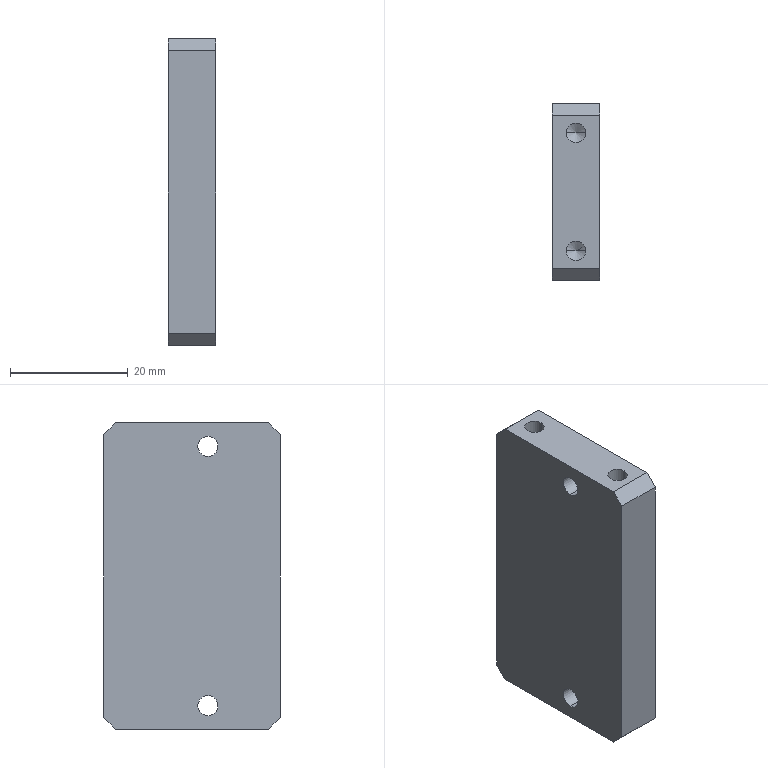Part | STEP file | 11-FG-S02311 | 1 solid | 36 faces | box 8 x 30 x 52 mm | volume 11750 mm3 | cylinder 16 | plane 12 | cone 8 | commonest cylinder face diameters 3.3 x8 3.4 x4 6.5 x4
STEP:
#1=CARTESIAN_POINT('',(-1.65,10.,15.9));
#2=VERTEX_POINT('',#1);
#3=CARTESIAN_POINT('',(1.65,10.,15.9));
#4=VERTEX_POINT('',#3);
#5=CARTESIAN_POINT('',(0.,10.,15.9));
#6=DIRECTION('',(0.,0.,1.));
#7=DIRECTION('',(1.,0.,0.));
#8=AXIS2_PLACEMENT_3D('',#5,#6,#7);
#9=CIRCLE('',#8,1.65);
#10=EDGE_CURVE('',#2,#4,#9,.T.);
#11=ORIENTED_EDGE('',*,*,#10,.F.);
#12=CARTESIAN_POINT('',(-1.65,10.,26.));
#13=VERTEX_POINT('',#12);
#14=CARTESIAN_POINT('',(-1.65,10.,26.));
#15=DIRECTION('',(0.,0.,1.));
#16=VECTOR('',#15,1000.);
#17=LINE('',#14,#16);
#18=EDGE_CURVE('',#2,#13,#17,.T.);
#19=ORIENTED_EDGE('',*,*,#18,.T.);
#20=CARTESIAN_POINT('',(1.65,10.,26.));
#21=VERTEX_POINT('',#20);
#22=CARTESIAN_POINT('',(0.,10.,26.));
#23=DIRECTION('',(0.,0.,1.));
#24=DIRECTION('',(1.,0.,0.));
#25=AXIS2_PLACEMENT_3D('',#22,#23,#24);
#26=CIRCLE('',#25,1.65);
#27=EDGE_CURVE('',#13,#21,#26,.T.);
#28=ORIENTED_EDGE('',*,*,#27,.T.);
#29=CARTESIAN_POINT('',(1.65,10.,26.));
#30=DIRECTION('',(0.,0.,1.));
#31=VECTOR('',#30,1000.);
#32=LINE('',#29,#31);
#33=EDGE_CURVE('',#4,#21,#32,.T.);
#34=ORIENTED_EDGE('',*,*,#33,.F.);
#35=EDGE_LOOP('',(#11,#19,#28,#34));
#36=FACE_OUTER_BOUND('',#35,.T.);
#37=CARTESIAN_POINT('',(0.,10.,26.));
#38=DIRECTION('',(0.,0.,1.));
#39=DIRECTION('',(1.,0.,0.));
#40=AXIS2_PLACEMENT_3D('',#37,#38,#39);
#41=CYLINDRICAL_SURFACE('',#40,1.65);
#42=ADVANCED_FACE('',(#36),#41,.F.);
#43=CARTESIAN_POINT('',(0.,10.,14.909));
#44=VERTEX_POINT('',#43);
#45=CARTESIAN_POINT('',(1.65,10.,15.9));
#46=DIRECTION('',(0.8572,0.,0.515));
#47=VECTOR('',#46,1000.);
#48=LINE('',#45,#47);
#49=EDGE_CURVE('',#44,#4,#48,.T.);
#50=ORIENTED_EDGE('',*,*,#49,.F.);
#51=CARTESIAN_POINT('',(-1.65,10.,15.9));
#52=DIRECTION('',(-0.8572,0.,0.515));
#53=VECTOR('',#52,1000.);
#54=LINE('',#51,#53);
#55=EDGE_CURVE('',#44,#2,#54,.T.);
#56=ORIENTED_EDGE('',*,*,#55,.T.);
#57=ORIENTED_EDGE('',*,*,#10,.T.);
#58=EDGE_LOOP('',(#50,#56,#57));
#59=FACE_OUTER_BOUND('',#58,.T.);
#60=CARTESIAN_POINT('',(0.,10.,15.9));
#61=DIRECTION('',(0.,0.,1.));
#62=DIRECTION('',(1.,0.,0.));
#63=AXIS2_PLACEMENT_3D('',#60,#61,#62);
#64=CONICAL_SURFACE('',#63,1.65,1.03);
#65=ADVANCED_FACE('',(#59),#64,.F.);
#66=CARTESIAN_POINT('',(-1.65,-10.,15.9));
#67=VERTEX_POINT('',#66);
#68=CARTESIAN_POINT('',(1.65,-10.,15.9));
#69=VERTEX_POINT('',#68);
#70=CARTESIAN_POINT('',(0.,-10.,15.9));
#71=DIRECTION('',(0.,0.,1.));
#72=DIRECTION('',(1.,0.,0.));
#73=AXIS2_PLACEMENT_3D('',#70,#71,#72);
#74=CIRCLE('',#73,1.65);
#75=EDGE_CURVE('',#67,#69,#74,.T.);
#76=ORIENTED_EDGE('',*,*,#75,.F.);
#77=CARTESIAN_POINT('',(-1.65,-10.,26.));
#78=VERTEX_POINT('',#77);
#79=CARTESIAN_POINT('',(-1.65,-10.,26.));
#80=DIRECTION('',(0.,0.,1.));
#81=VECTOR('',#80,1000.);
#82=LINE('',#79,#81);
#83=EDGE_CURVE('',#67,#78,#82,.T.);
#84=ORIENTED_EDGE('',*,*,#83,.T.);
#85=CARTESIAN_POINT('',(1.65,-10.,26.));
#86=VERTEX_POINT('',#85);
#87=CARTESIAN_POINT('',(0.,-10.,26.));
#88=DIRECTION('',(0.,0.,1.));
#89=DIRECTION('',(1.,0.,0.));
#90=AXIS2_PLACEMENT_3D('',#87,#88,#89);
#91=CIRCLE('',#90,1.65);
#92=EDGE_CURVE('',#78,#86,#91,.T.);
#93=ORIENTED_EDGE('',*,*,#92,.T.);
#94=CARTESIAN_POINT('',(1.65,-10.,26.));
#95=DIRECTION('',(0.,0.,1.));
#96=VECTOR('',#95,1000.);
#97=LINE('',#94,#96);
#98=EDGE_CURVE('',#69,#86,#97,.T.);
#99=ORIENTED_EDGE('',*,*,#98,.F.);
#100=EDGE_LOOP('',(#76,#84,#93,#99));
#101=FACE_OUTER_BOUND('',#100,.T.);
#102=CARTESIAN_POINT('',(0.,-10.,26.));
#103=DIRECTION('',(0.,0.,1.));
#104=DIRECTION('',(1.,0.,0.));
#105=AXIS2_PLACEMENT_3D('',#102,#103,#104);
#106=CYLINDRICAL_SURFACE('',#105,1.65);
#107=ADVANCED_FACE('',(#101),#106,.F.);
#108=CARTESIAN_POINT('',(0.,-10.,14.909));
#109=VERTEX_POINT('',#108);
#110=CARTESIAN_POINT('',(1.65,-10.,15.9));
#111=DIRECTION('',(0.8572,0.,0.515));
#112=VECTOR('',#111,1000.);
#113=LINE('',#110,#112);
#114=EDGE_CURVE('',#109,#69,#113,.T.);
#115=ORIENTED_EDGE('',*,*,#114,.F.);
#116=CARTESIAN_POINT('',(-1.65,-10.,15.9));
#117=DIRECTION('',(-0.8572,0.,0.515));
#118=VECTOR('',#117,1000.);
#119=LINE('',#116,#118);
#120=EDGE_CURVE('',#109,#67,#119,.T.);
#121=ORIENTED_EDGE('',*,*,#120,.T.);
#122=ORIENTED_EDGE('',*,*,#75,.T.);
#123=EDGE_LOOP('',(#115,#121,#122));
#124=FACE_OUTER_BOUND('',#123,.T.);
#125=CARTESIAN_POINT('',(0.,-10.,15.9));
#126=DIRECTION('',(0.,0.,1.));
#127=DIRECTION('',(1.,0.,0.));
#128=AXIS2_PLACEMENT_3D('',#125,#126,#127);
#129=CONICAL_SURFACE('',#128,1.65,1.03);
#130=ADVANCED_FACE('',(#124),#129,.F.);
#131=CARTESIAN_POINT('',(1.65,10.,-15.9));
#132=VERTEX_POINT('',#131);
#133=CARTESIAN_POINT('',(-1.65,10.,-15.9));
#134=VERTEX_POINT('',#133);
#135=CARTESIAN_POINT('',(0.,10.,-15.9));
#136=DIRECTION('',(0.,0.,-1.));
#137=DIRECTION('',(-1.,0.,0.));
#138=AXIS2_PLACEMENT_3D('',#135,#136,#137);
#139=CIRCLE('',#138,1.65);
#140=EDGE_CURVE('',#132,#134,#139,.T.);
#141=ORIENTED_EDGE('',*,*,#140,.F.);
#142=CARTESIAN_POINT('',(1.65,10.,-26.));
#143=VERTEX_POINT('',#142);
#144=CARTESIAN_POINT('',(1.65,10.,-26.));
#145=DIRECTION('',(0.,0.,-1.));
#146=VECTOR('',#145,1000.);
#147=LINE('',#144,#146);
#148=EDGE_CURVE('',#132,#143,#147,.T.);
#149=ORIENTED_EDGE('',*,*,#148,.T.);
#150=CARTESIAN_POINT('',(-1.65,10.,-26.));
#151=VERTEX_POINT('',#150);
#152=CARTESIAN_POINT('',(0.,10.,-26.));
#153=DIRECTION('',(0.,0.,-1.));
#154=DIRECTION('',(-1.,0.,0.));
#155=AXIS2_PLACEMENT_3D('',#152,#153,#154);
#156=CIRCLE('',#155,1.65);
#157=EDGE_CURVE('',#143,#151,#156,.T.);
#158=ORIENTED_EDGE('',*,*,#157,.T.);
#159=CARTESIAN_POINT('',(-1.65,10.,-26.));
#160=DIRECTION('',(0.,0.,-1.));
#161=VECTOR('',#160,1000.);
#162=LINE('',#159,#161);
#163=EDGE_CURVE('',#134,#151,#162,.T.);
#164=ORIENTED_EDGE('',*,*,#163,.F.);
#165=EDGE_LOOP('',(#141,#149,#158,#164));
#166=FACE_OUTER_BOUND('',#165,.T.);
#167=CARTESIAN_POINT('',(0.,10.,-26.));
#168=DIRECTION('',(0.,0.,-1.));
#169=DIRECTION('',(-1.,0.,0.));
#170=AXIS2_PLACEMENT_3D('',#167,#168,#169);
#171=CYLINDRICAL_SURFACE('',#170,1.65);
#172=ADVANCED_FACE('',(#166),#171,.F.);
#173=CARTESIAN_POINT('',(0.,10.,-14.909));
#174=VERTEX_POINT('',#173);
#175=CARTESIAN_POINT('',(-1.65,10.,-15.9));
#176=DIRECTION('',(-0.8572,0.,-0.515));
#177=VECTOR('',#176,1000.);
#178=LINE('',#175,#177);
#179=EDGE_CURVE('',#174,#134,#178,.T.);
#180=ORIENTED_EDGE('',*,*,#179,.F.);
#181=CARTESIAN_POINT('',(1.65,10.,-15.9));
#182=DIRECTION('',(0.8572,0.,-0.515));
#183=VECTOR('',#182,1000.);
#184=LINE('',#181,#183);
#185=EDGE_CURVE('',#174,#132,#184,.T.);
#186=ORIENTED_EDGE('',*,*,#185,.T.);
#187=ORIENTED_EDGE('',*,*,#140,.T.);
#188=EDGE_LOOP('',(#180,#186,#187));
#189=FACE_OUTER_BOUND('',#188,.T.);
#190=CARTESIAN_POINT('',(0.,10.,-15.9));
#191=DIRECTION('',(0.,0.,-1.));
#192=DIRECTION('',(-1.,0.,0.));
#193=AXIS2_PLACEMENT_3D('',#190,#191,#192);
#194=CONICAL_SURFACE('',#193,1.65,1.03);
#195=ADVANCED_FACE('',(#189),#194,.F.);
#196=CARTESIAN_POINT('',(1.65,-10.,-15.9));
#197=VERTEX_POINT('',#196);
#198=CARTESIAN_POINT('',(-1.65,-10.,-15.9));
#199=VERTEX_POINT('',#198);
#200=CARTESIAN_POINT('',(0.,-10.,-15.9));
#201=DIRECTION('',(0.,0.,-1.));
#202=DIRECTION('',(-1.,0.,0.));
#203=AXIS2_PLACEMENT_3D('',#200,#201,#202);
#204=CIRCLE('',#203,1.65);
#205=EDGE_CURVE('',#197,#199,#204,.T.);
#206=ORIENTED_EDGE('',*,*,#205,.F.);
#207=CARTESIAN_POINT('',(1.65,-10.,-26.));
#208=VERTEX_POINT('',#207);
#209=CARTESIAN_POINT('',(1.65,-10.,-26.));
#210=DIRECTION('',(0.,0.,-1.));
#211=VECTOR('',#210,1000.);
#212=LINE('',#209,#211);
#213=EDGE_CURVE('',#197,#208,#212,.T.);
#214=ORIENTED_EDGE('',*,*,#213,.T.);
#215=CARTESIAN_POINT('',(-1.65,-10.,-26.));
#216=VERTEX_POINT('',#215);
#217=CARTESIAN_POINT('',(0.,-10.,-26.));
#218=DIRECTION('',(0.,0.,-1.));
#219=DIRECTION('',(-1.,0.,0.));
#220=AXIS2_PLACEMENT_3D('',#217,#218,#219);
#221=CIRCLE('',#220,1.65);
#222=EDGE_CURVE('',#208,#216,#221,.T.);
#223=ORIENTED_EDGE('',*,*,#222,.T.);
#224=CARTESIAN_POINT('',(-1.65,-10.,-26.));
#225=DIRECTION('',(0.,0.,-1.));
#226=VECTOR('',#225,1000.);
#227=LINE('',#224,#226);
#228=EDGE_CURVE('',#199,#216,#227,.T.);
#229=ORIENTED_EDGE('',*,*,#228,.F.);
#230=EDGE_LOOP('',(#206,#214,#223,#229));
#231=FACE_OUTER_BOUND('',#230,.T.);
#232=CARTESIAN_POINT('',(0.,-10.,-26.));
#233=DIRECTION('',(0.,0.,-1.));
#234=DIRECTION('',(-1.,0.,0.));
#235=AXIS2_PLACEMENT_3D('',#232,#233,#234);
#236=CYLINDRICAL_SURFACE('',#235,1.65);
#237=ADVANCED_FACE('',(#231),#236,.F.);
#238=CARTESIAN_POINT('',(0.,-10.,-14.909));
#239=VERTEX_POINT('',#238);
#240=CARTESIAN_POINT('',(-1.65,-10.,-15.9));
#241=DIRECTION('',(-0.8572,0.,-0.515));
#242=VECTOR('',#241,1000.);
#243=LINE('',#240,#242);
#244=EDGE_CURVE('',#239,#199,#243,.T.);
#245=ORIENTED_EDGE('',*,*,#244,.F.);
#246=CARTESIAN_POINT('',(1.65,-10.,-15.9));
#247=DIRECTION('',(0.8572,0.,-0.515));
#248=VECTOR('',#247,1000.);
#249=LINE('',#246,#248);
#250=EDGE_CURVE('',#239,#197,#249,.T.);
#251=ORIENTED_EDGE('',*,*,#250,.T.);
#252=ORIENTED_EDGE('',*,*,#205,.T.);
#253=EDGE_LOOP('',(#245,#251,#252));
#254=FACE_OUTER_BOUND('',#253,.T.);
#255=CARTESIAN_POINT('',(0.,-10.,-15.9));
#256=DIRECTION('',(0.,0.,-1.));
#257=DIRECTION('',(-1.,0.,0.));
#258=AXIS2_PLACEMENT_3D('',#255,#256,#257);
#259=CONICAL_SURFACE('',#258,1.65,1.03);
#260=ADVANCED_FACE('',(#254),#259,.F.);
#261=CARTESIAN_POINT('',(0.6,-2.7,-18.75));
#262=VERTEX_POINT('',#261);
#263=CARTESIAN_POINT('',(0.6,-2.7,-25.25));
#264=VERTEX_POINT('',#263);
#265=CARTESIAN_POINT('',(0.6,-2.7,-22.));
#266=DIRECTION('',(1.,0.,0.));
#267=DIRECTION('',(0.,0.,-1.));
#268=AXIS2_PLACEMENT_3D('',#265,#266,#267);
#269=CIRCLE('',#268,3.25);
#270=EDGE_CURVE('',#262,#264,#269,.T.);
#271=ORIENTED_EDGE('',*,*,#270,.F.);
#272=CARTESIAN_POINT('',(4.,-2.7,-18.75));
#273=VERTEX_POINT('',#272);
#274=CARTESIAN_POINT('',(4.,-2.7,-18.75));
#275=DIRECTION('',(1.,0.,0.));
#276=VECTOR('',#275,1000.);
#277=LINE('',#274,#276);
#278=EDGE_CURVE('',#262,#273,#277,.T.);
#279=ORIENTED_EDGE('',*,*,#278,.T.);
#280=CARTESIAN_POINT('',(4.,-2.7,-25.25));
#281=VERTEX_POINT('',#280);
#282=CARTESIAN_POINT('',(4.,-2.7,-22.));
#283=DIRECTION('',(1.,0.,0.));
#284=DIRECTION('',(0.,0.,-1.));
#285=AXIS2_PLACEMENT_3D('',#282,#283,#284);
#286=CIRCLE('',#285,3.25);
#287=EDGE_CURVE('',#273,#281,#286,.T.);
#288=ORIENTED_EDGE('',*,*,#287,.T.);
#289=CARTESIAN_POINT('',(4.,-2.7,-25.25));
#290=DIRECTION('',(1.,0.,0.));
#291=VECTOR('',#290,1000.);
#292=LINE('',#289,#291);
#293=EDGE_CURVE('',#264,#281,#292,.T.);
#294=ORIENTED_EDGE('',*,*,#293,.F.);
#295=EDGE_LOOP('',(#271,#279,#288,#294));
#296=FACE_OUTER_BOUND('',#295,.T.);
#297=CARTESIAN_POINT('',(4.,-2.7,-22.));
#298=DIRECTION('',(1.,0.,0.));
#299=DIRECTION('',(0.,0.,-1.));
#300=AXIS2_PLACEMENT_3D('',#297,#298,#299);
#301=CYLINDRICAL_SURFACE('',#300,3.25);
#302=ADVANCED_FACE('',(#296),#301,.F.);
#303=CARTESIAN_POINT('',(-4.,-2.7,-20.3));
#304=VERTEX_POINT('',#303);
#305=CARTESIAN_POINT('',(-4.,-2.7,-23.7));
#306=VERTEX_POINT('',#305);
#307=CARTESIAN_POINT('',(-4.,-2.7,-22.));
#308=DIRECTION('',(1.,0.,0.));
#309=DIRECTION('',(0.,0.,-1.));
#310=AXIS2_PLACEMENT_3D('',#307,#308,#309);
#311=CIRCLE('',#310,1.7);
#312=EDGE_CURVE('',#304,#306,#311,.T.);
#313=ORIENTED_EDGE('',*,*,#312,.F.);
#314=CARTESIAN_POINT('',(0.6,-2.7,-20.3));
#315=VERTEX_POINT('',#314);
#316=CARTESIAN_POINT('',(4.,-2.7,-20.3));
#317=DIRECTION('',(1.,0.,0.));
#318=VECTOR('',#317,1000.);
#319=LINE('',#316,#318);
#320=EDGE_CURVE('',#304,#315,#319,.T.);
#321=ORIENTED_EDGE('',*,*,#320,.T.);
#322=CARTESIAN_POINT('',(0.6,-2.7,-23.7));
#323=VERTEX_POINT('',#322);
#324=CARTESIAN_POINT('',(0.6,-2.7,-22.));
#325=DIRECTION('',(1.,0.,0.));
#326=DIRECTION('',(0.,0.,-1.));
#327=AXIS2_PLACEMENT_3D('',#324,#325,#326);
#328=CIRCLE('',#327,1.7);
#329=EDGE_CURVE('',#315,#323,#328,.T.);
#330=ORIENTED_EDGE('',*,*,#329,.T.);
#331=CARTESIAN_POINT('',(4.,-2.7,-23.7));
#332=DIRECTION('',(1.,0.,0.));
#333=VECTOR('',#332,1000.);
#334=LINE('',#331,#333);
#335=EDGE_CURVE('',#306,#323,#334,.T.);
#336=ORIENTED_EDGE('',*,*,#335,.F.);
#337=EDGE_LOOP('',(#313,#321,#330,#336));
#338=FACE_OUTER_BOUND('',#337,.T.);
#339=CARTESIAN_POINT('',(4.,-2.7,-22.));
#340=DIRECTION('',(1.,0.,0.));
#341=DIRECTION('',(0.,0.,-1.));
#342=AXIS2_PLACEMENT_3D('',#339,#340,#341);
#343=CYLINDRICAL_SURFACE('',#342,1.7);
#344=ADVANCED_FACE('',(#338),#343,.F.);
#345=CARTESIAN_POINT('',(0.6,-2.7,25.25));
#346=VERTEX_POINT('',#345);
#347=CARTESIAN_POINT('',(0.6,-2.7,18.75));
#348=VERTEX_POINT('',#347);
#349=CARTESIAN_POINT('',(0.6,-2.7,22.));
#350=DIRECTION('',(1.,0.,0.));
#351=DIRECTION('',(0.,0.,-1.));
#352=AXIS2_PLACEMENT_3D('',#349,#350,#351);
#353=CIRCLE('',#352,3.25);
#354=EDGE_CURVE('',#346,#348,#353,.T.);
#355=ORIENTED_EDGE('',*,*,#354,.F.);
#356=CARTESIAN_POINT('',(4.,-2.7,25.25));
#357=VERTEX_POINT('',#356);
#358=CARTESIAN_POINT('',(4.,-2.7,25.25));
#359=DIRECTION('',(1.,0.,0.));
#360=VECTOR('',#359,1000.);
#361=LINE('',#358,#360);
#362=EDGE_CURVE('',#346,#357,#361,.T.);
#363=ORIENTED_EDGE('',*,*,#362,.T.);
#364=CARTESIAN_POINT('',(4.,-2.7,18.75));
#365=VERTEX_POINT('',#364);
#366=CARTESIAN_POINT('',(4.,-2.7,22.));
#367=DIRECTION('',(1.,0.,0.));
#368=DIRECTION('',(0.,0.,-1.));
#369=AXIS2_PLACEMENT_3D('',#366,#367,#368);
#370=CIRCLE('',#369,3.25);
#371=EDGE_CURVE('',#357,#365,#370,.T.);
#372=ORIENTED_EDGE('',*,*,#371,.T.);
#373=CARTESIAN_POINT('',(4.,-2.7,18.75));
#374=DIRECTION('',(1.,0.,0.));
#375=VECTOR('',#374,1000.);
#376=LINE('',#373,#375);
#377=EDGE_CURVE('',#348,#365,#376,.T.);
#378=ORIENTED_EDGE('',*,*,#377,.F.);
#379=EDGE_LOOP('',(#355,#363,#372,#378));
#380=FACE_OUTER_BOUND('',#379,.T.);
#381=CARTESIAN_POINT('',(4.,-2.7,22.));
#382=DIRECTION('',(1.,0.,0.));
#383=DIRECTION('',(0.,0.,-1.));
#384=AXIS2_PLACEMENT_3D('',#381,#382,#383);
#385=CYLINDRICAL_SURFACE('',#384,3.25);
#386=ADVANCED_FACE('',(#380),#385,.F.);
#387=CARTESIAN_POINT('',(-4.,-2.7,23.7));
#388=VERTEX_POINT('',#387);
#389=CARTESIAN_POINT('',(-4.,-2.7,20.3));
#390=VERTEX_POINT('',#389);
#391=CARTESIAN_POINT('',(-4.,-2.7,22.));
#392=DIRECTION('',(1.,0.,0.));
#393=DIRECTION('',(0.,0.,-1.));
#394=AXIS2_PLACEMENT_3D('',#391,#392,#393);
#395=CIRCLE('',#394,1.7);
#396=EDGE_CURVE('',#388,#390,#395,.T.);
#397=ORIENTED_EDGE('',*,*,#396,.F.);
#398=CARTESIAN_POINT('',(0.6,-2.7,23.7));
#399=VERTEX_POINT('',#398);
#400=CARTESIAN_POINT('',(4.,-2.7,23.7));
#401=DIRECTION('',(1.,0.,0.));
#402=VECTOR('',#401,1000.);
#403=LINE('',#400,#402);
#404=EDGE_CURVE('',#388,#399,#403,.T.);
#405=ORIENTED_EDGE('',*,*,#404,.T.);
#406=CARTESIAN_POINT('',(0.6,-2.7,20.3));
#407=VERTEX_POINT('',#406);
#408=CARTESIAN_POINT('',(0.6,-2.7,22.));
#409=DIRECTION('',(1.,0.,0.));
#410=DIRECTION('',(0.,0.,-1.));
#411=AXIS2_PLACEMENT_3D('',#408,#409,#410);
#412=CIRCLE('',#411,1.7);
#413=EDGE_CURVE('',#399,#407,#412,.T.);
#414=ORIENTED_EDGE('',*,*,#413,.T.);
#415=CARTESIAN_POINT('',(4.,-2.7,20.3));
#416=DIRECTION('',(1.,0.,0.));
#417=VECTOR('',#416,1000.);
#418=LINE('',#415,#417);
#419=EDGE_CURVE('',#390,#407,#418,.T.);
#420=ORIENTED_EDGE('',*,*,#419,.F.);
#421=EDGE_LOOP('',(#397,#405,#414,#420));
#422=FACE_OUTER_BOUND('',#421,.T.);
#423=CARTESIAN_POINT('',(4.,-2.7,22.));
#424=DIRECTION('',(1.,0.,0.));
#425=DIRECTION('',(0.,0.,-1.));
#426=AXIS2_PLACEMENT_3D('',#423,#424,#425);
#427=CYLINDRICAL_SURFACE('',#426,1.7);
#428=ADVANCED_FACE('',(#422),#427,.F.);
#429=CARTESIAN_POINT('',(4.,-2.7,-22.));
#430=DIRECTION('',(1.,0.,0.));
#431=DIRECTION('',(0.,0.,-1.));
#432=AXIS2_PLACEMENT_3D('',#429,#430,#431);
#433=CIRCLE('',#432,3.25);
#434=EDGE_CURVE('',#281,#273,#433,.T.);
#435=ORIENTED_EDGE('',*,*,#434,.F.);
#436=ORIENTED_EDGE('',*,*,#287,.F.);
#437=EDGE_LOOP('',(#435,#436));
#438=FACE_BOUND('',#437,.T.);
#439=CARTESIAN_POINT('',(4.,-2.7,22.));
#440=DIRECTION('',(1.,0.,0.));
#441=DIRECTION('',(0.,0.,-1.));
#442=AXIS2_PLACEMENT_3D('',#439,#440,#441);
#443=CIRCLE('',#442,3.25);
#444=EDGE_CURVE('',#365,#357,#443,.T.);
#445=ORIENTED_EDGE('',*,*,#444,.F.);
#446=ORIENTED_EDGE('',*,*,#371,.F.);
#447=EDGE_LOOP('',(#445,#446));
#448=FACE_BOUND('',#447,.T.);
#449=CARTESIAN_POINT('',(4.,15.,24.));
#450=VERTEX_POINT('',#449);
#451=CARTESIAN_POINT('',(4.,15.,-24.));
#452=VERTEX_POINT('',#451);
#453=CARTESIAN_POINT('',(4.,15.,26.));
#454=DIRECTION('',(0.,0.,-1.));
#455=VECTOR('',#454,1000.);
#456=LINE('',#453,#455);
#457=EDGE_CURVE('',#450,#452,#456,.T.);
#458=ORIENTED_EDGE('',*,*,#457,.F.);
#459=CARTESIAN_POINT('',(4.,13.,26.));
#460=VERTEX_POINT('',#459);
#461=CARTESIAN_POINT('',(4.,13.,26.));
#462=DIRECTION('',(0.,-0.7071,0.7071));
#463=VECTOR('',#462,1000.);
#464=LINE('',#461,#463);
#465=EDGE_CURVE('',#450,#460,#464,.T.);
#466=ORIENTED_EDGE('',*,*,#465,.T.);
#467=CARTESIAN_POINT('',(4.,-13.,26.));
#468=VERTEX_POINT('',#467);
#469=CARTESIAN_POINT('',(4.,-15.,26.));
#470=DIRECTION('',(0.,1.,0.));
#471=VECTOR('',#470,1000.);
#472=LINE('',#469,#471);
#473=EDGE_CURVE('',#468,#460,#472,.T.);
#474=ORIENTED_EDGE('',*,*,#473,.F.);
#475=CARTESIAN_POINT('',(4.,-15.,24.));
#476=VERTEX_POINT('',#475);
#477=CARTESIAN_POINT('',(4.,-13.,26.));
#478=DIRECTION('',(0.,-0.7071,-0.7071));
#479=VECTOR('',#478,1000.);
#480=LINE('',#477,#479);
#481=EDGE_CURVE('',#468,#476,#480,.T.);
#482=ORIENTED_EDGE('',*,*,#481,.T.);
#483=CARTESIAN_POINT('',(4.,-15.,-24.));
#484=VERTEX_POINT('',#483);
#485=CARTESIAN_POINT('',(4.,-15.,26.));
#486=DIRECTION('',(0.,0.,-1.));
#487=VECTOR('',#486,1000.);
#488=LINE('',#485,#487);
#489=EDGE_CURVE('',#476,#484,#488,.T.);
#490=ORIENTED_EDGE('',*,*,#489,.T.);
#491=CARTESIAN_POINT('',(4.,-13.,-26.));
#492=VERTEX_POINT('',#491);
#493=CARTESIAN_POINT('',(4.,-15.,-24.));
#494=DIRECTION('',(0.,0.7071,-0.7071));
#495=VECTOR('',#494,1000.);
#496=LINE('',#493,#495);
#497=EDGE_CURVE('',#484,#492,#496,.T.);
#498=ORIENTED_EDGE('',*,*,#497,.T.);
#499=CARTESIAN_POINT('',(4.,13.,-26.));
#500=VERTEX_POINT('',#499);
#501=CARTESIAN_POINT('',(4.,-15.,-26.));
#502=DIRECTION('',(0.,1.,0.));
#503=VECTOR('',#502,1000.);
#504=LINE('',#501,#503);
#505=EDGE_CURVE('',#492,#500,#504,.T.);
#506=ORIENTED_EDGE('',*,*,#505,.T.);
#507=CARTESIAN_POINT('',(4.,15.,-24.));
#508=DIRECTION('',(0.,0.7071,0.7071));
#509=VECTOR('',#508,1000.);
#510=LINE('',#507,#509);
#511=EDGE_CURVE('',#500,#452,#510,.T.);
#512=ORIENTED_EDGE('',*,*,#511,.T.);
#513=EDGE_LOOP('',(#458,#466,#474,#482,#490,#498,#506,#512));
#514=FACE_OUTER_BOUND('',#513,.T.);
#515=CARTESIAN_POINT('',(4.,-15.,26.));
#516=DIRECTION('',(-1.,0.,0.));
#517=DIRECTION('',(0.,0.,1.));
#518=AXIS2_PLACEMENT_3D('',#515,#516,#517);
#519=PLANE('',#518);
#520=ADVANCED_FACE('',(#438,#448,#514),#519,.F.);
#521=CARTESIAN_POINT('',(-4.,15.,24.));
#522=VERTEX_POINT('',#521);
#523=CARTESIAN_POINT('',(-4.,15.,-24.));
#524=VERTEX_POINT('',#523);
#525=CARTESIAN_POINT('',(-4.,15.,26.));
#526=DIRECTION('',(0.,0.,-1.));
#527=VECTOR('',#526,1000.);
#528=LINE('',#525,#527);
#529=EDGE_CURVE('',#522,#524,#528,.T.);
#530=ORIENTED_EDGE('',*,*,#529,.F.);
#531=CARTESIAN_POINT('',(-4.,15.,24.));
#532=DIRECTION('',(1.,0.,0.));
#533=VECTOR('',#532,1000.);
#534=LINE('',#531,#533);
#535=EDGE_CURVE('',#522,#450,#534,.T.);
#536=ORIENTED_EDGE('',*,*,#535,.T.);
#537=ORIENTED_EDGE('',*,*,#457,.T.);
#538=CARTESIAN_POINT('',(-4.,15.,-24.));
#539=DIRECTION('',(-1.,0.,0.));
#540=VECTOR('',#539,1000.);
#541=LINE('',#538,#540);
#542=EDGE_CURVE('',#452,#524,#541,.T.);
#543=ORIENTED_EDGE('',*,*,#542,.T.);
#544=EDGE_LOOP('',(#530,#536,#537,#543));
#545=FACE_OUTER_BOUND('',#544,.T.);
#546=CARTESIAN_POINT('',(-4.,15.,26.));
#547=DIRECTION('',(0.,-1.,0.));
#548=DIRECTION('',(0.,0.,-1.));
#549=AXIS2_PLACEMENT_3D('',#546,#547,#548);
#550=PLANE('',#549);
#551=ADVANCED_FACE('',(#545),#550,.F.);
#552=CARTESIAN_POINT('',(-4.,-2.7,-22.));
#553=DIRECTION('',(1.,0.,0.));
#554=DIRECTION('',(0.,0.,-1.));
#555=AXIS2_PLACEMENT_3D('',#552,#553,#554);
#556=CIRCLE('',#555,1.7);
#557=EDGE_CURVE('',#306,#304,#556,.T.);
#558=ORIENTED_EDGE('',*,*,#557,.T.);
#559=ORIENTED_EDGE('',*,*,#312,.T.);
#560=EDGE_LOOP('',(#558,#559));
#561=FACE_BOUND('',#560,.T.);
#562=CARTESIAN_POINT('',(-4.,-2.7,22.));
#563=DIRECTION('',(1.,0.,0.));
#564=DIRECTION('',(0.,0.,-1.));
#565=AXIS2_PLACEMENT_3D('',#562,#563,#564);
#566=CIRCLE('',#565,1.7);
#567=EDGE_CURVE('',#390,#388,#566,.T.);
#568=ORIENTED_EDGE('',*,*,#567,.T.);
#569=ORIENTED_EDGE('',*,*,#396,.T.);
#570=EDGE_LOOP('',(#568,#569));
#571=FACE_BOUND('',#570,.T.);
#572=CARTESIAN_POINT('',(-4.,13.,26.));
#573=VERTEX_POINT('',#572);
#574=CARTESIAN_POINT('',(-4.,-13.,26.));
#575=VERTEX_POINT('',#574);
#576=CARTESIAN_POINT('',(-4.,-15.,26.));
#577=DIRECTION('',(0.,-1.,0.));
#578=VECTOR('',#577,1000.);
#579=LINE('',#576,#578);
#580=EDGE_CURVE('',#573,#575,#579,.T.);
#581=ORIENTED_EDGE('',*,*,#580,.F.);
#582=CARTESIAN_POINT('',(-4.,13.,26.));
#583=DIRECTION('',(0.,0.7071,-0.7071));
#584=VECTOR('',#583,1000.);
#585=LINE('',#582,#584);
#586=EDGE_CURVE('',#573,#522,#585,.T.);
#587=ORIENTED_EDGE('',*,*,#586,.T.);
#588=ORIENTED_EDGE('',*,*,#529,.T.);
#589=CARTESIAN_POINT('',(-4.,13.,-26.));
#590=VERTEX_POINT('',#589);
#591=CARTESIAN_POINT('',(-4.,15.,-24.));
#592=DIRECTION('',(0.,-0.7071,-0.7071));
#593=VECTOR('',#592,1000.);
#594=LINE('',#591,#593);
#595=EDGE_CURVE('',#524,#590,#594,.T.);
#596=ORIENTED_EDGE('',*,*,#595,.T.);
#597=CARTESIAN_POINT('',(-4.,-13.,-26.));
#598=VERTEX_POINT('',#597);
#599=CARTESIAN_POINT('',(-4.,-15.,-26.));
#600=DIRECTION('',(0.,-1.,0.));
#601=VECTOR('',#600,1000.);
#602=LINE('',#599,#601);
#603=EDGE_CURVE('',#590,#598,#602,.T.);
#604=ORIENTED_EDGE('',*,*,#603,.T.);
#605=CARTESIAN_POINT('',(-4.,-15.,-24.));
#606=VERTEX_POINT('',#605);
#607=CARTESIAN_POINT('',(-4.,-15.,-24.));
#608=DIRECTION('',(0.,-0.7071,0.7071));
#609=VECTOR('',#608,1000.);
#610=LINE('',#607,#609);
#611=EDGE_CURVE('',#598,#606,#610,.T.);
#612=ORIENTED_EDGE('',*,*,#611,.T.);
#613=CARTESIAN_POINT('',(-4.,-15.,24.));
#614=VERTEX_POINT('',#613);
#615=CARTESIAN_POINT('',(-4.,-15.,26.));
#616=DIRECTION('',(0.,0.,-1.));
#617=VECTOR('',#616,1000.);
#618=LINE('',#615,#617);
#619=EDGE_CURVE('',#614,#606,#618,.T.);
#620=ORIENTED_EDGE('',*,*,#619,.F.);
#621=CARTESIAN_POINT('',(-4.,-13.,26.));
#622=DIRECTION('',(0.,0.7071,0.7071));
#623=VECTOR('',#622,1000.);
#624=LINE('',#621,#623);
#625=EDGE_CURVE('',#614,#575,#624,.T.);
#626=ORIENTED_EDGE('',*,*,#625,.T.);
#627=EDGE_LOOP('',(#581,#587,#588,#596,#604,#612,#620,#626));
#628=FACE_OUTER_BOUND('',#627,.T.);
#629=CARTESIAN_POINT('',(-4.,-15.,26.));
#630=DIRECTION('',(1.,0.,0.));
#631=DIRECTION('',(0.,0.,-1.));
#632=AXIS2_PLACEMENT_3D('',#629,#630,#631);
#633=PLANE('',#632);
#634=ADVANCED_FACE('',(#561,#571,#628),#633,.F.);
#635=ORIENTED_EDGE('',*,*,#489,.F.);
#636=CARTESIAN_POINT('',(-4.,-15.,24.));
#637=DIRECTION('',(-1.,0.,0.));
#638=VECTOR('',#637,1000.);
#639=LINE('',#636,#638);
#640=EDGE_CURVE('',#476,#614,#639,.T.);
#641=ORIENTED_EDGE('',*,*,#640,.T.);
#642=ORIENTED_EDGE('',*,*,#619,.T.);
#643=CARTESIAN_POINT('',(4.,-15.,-24.));
#644=DIRECTION('',(1.,0.,0.));
#645=VECTOR('',#644,1000.);
#646=LINE('',#643,#645);
#647=EDGE_CURVE('',#606,#484,#646,.T.);
#648=ORIENTED_EDGE('',*,*,#647,.T.);
#649=EDGE_LOOP('',(#635,#641,#642,#648));
#650=FACE_OUTER_BOUND('',#649,.T.);
#651=CARTESIAN_POINT('',(-4.,-15.,26.));
#652=DIRECTION('',(0.,1.,0.));
#653=DIRECTION('',(0.,0.,1.));
#654=AXIS2_PLACEMENT_3D('',#651,#652,#653);
#655=PLANE('',#654);
#656=ADVANCED_FACE('',(#650),#655,.F.);
#657=CARTESIAN_POINT('',(0.,10.,26.));
#658=DIRECTION('',(0.,0.,1.));
#659=DIRECTION('',(1.,0.,0.));
#660=AXIS2_PLACEMENT_3D('',#657,#658,#659);
#661=CIRCLE('',#660,1.65);
#662=EDGE_CURVE('',#21,#13,#661,.T.);
#663=ORIENTED_EDGE('',*,*,#662,.F.);
#664=ORIENTED_EDGE('',*,*,#27,.F.);
#665=EDGE_LOOP('',(#663,#664));
#666=FACE_BOUND('',#665,.T.);
#667=CARTESIAN_POINT('',(0.,-10.,26.));
#668=DIRECTION('',(0.,0.,1.));
#669=DIRECTION('',(1.,0.,0.));
#670=AXIS2_PLACEMENT_3D('',#667,#668,#669);
#671=CIRCLE('',#670,1.65);
#672=EDGE_CURVE('',#86,#78,#671,.T.);
#673=ORIENTED_EDGE('',*,*,#672,.F.);
#674=ORIENTED_EDGE('',*,*,#92,.F.);
#675=EDGE_LOOP('',(#673,#674));
#676=FACE_BOUND('',#675,.T.);
#677=ORIENTED_EDGE('',*,*,#473,.T.);
#678=CARTESIAN_POINT('',(0.,13.,26.));
#679=DIRECTION('',(-1.,0.,0.));
#680=VECTOR('',#679,1000.);
#681=LINE('',#678,#680);
#682=EDGE_CURVE('',#460,#573,#681,.T.);
#683=ORIENTED_EDGE('',*,*,#682,.T.);
#684=ORIENTED_EDGE('',*,*,#580,.T.);
#685=CARTESIAN_POINT('',(0.,-13.,26.));
#686=DIRECTION('',(1.,0.,0.));
#687=VECTOR('',#686,1000.);
#688=LINE('',#685,#687);
#689=EDGE_CURVE('',#575,#468,#688,.T.);
#690=ORIENTED_EDGE('',*,*,#689,.T.);
#691=EDGE_LOOP('',(#677,#683,#684,#690));
#692=FACE_OUTER_BOUND('',#691,.T.);
#693=CARTESIAN_POINT('',(0.,0.,26.));
#694=DIRECTION('',(0.,0.,-1.));
#695=DIRECTION('',(-1.,0.,0.));
#696=AXIS2_PLACEMENT_3D('',#693,#694,#695);
#697=PLANE('',#696);
#698=ADVANCED_FACE('',(#666,#676,#692),#697,.F.);
#699=CARTESIAN_POINT('',(0.,10.,-26.));
#700=DIRECTION('',(0.,0.,-1.));
#701=DIRECTION('',(-1.,0.,0.));
#702=AXIS2_PLACEMENT_3D('',#699,#700,#701);
#703=CIRCLE('',#702,1.65);
#704=EDGE_CURVE('',#151,#143,#703,.T.);
#705=ORIENTED_EDGE('',*,*,#704,.F.);
#706=ORIENTED_EDGE('',*,*,#157,.F.);
#707=EDGE_LOOP('',(#705,#706));
#708=FACE_BOUND('',#707,.T.);
#709=CARTESIAN_POINT('',(0.,-10.,-26.));
#710=DIRECTION('',(0.,0.,-1.));
#711=DIRECTION('',(-1.,0.,0.));
#712=AXIS2_PLACEMENT_3D('',#709,#710,#711);
#713=CIRCLE('',#712,1.65);
#714=EDGE_CURVE('',#216,#208,#713,.T.);
#715=ORIENTED_EDGE('',*,*,#714,.F.);
#716=ORIENTED_EDGE('',*,*,#222,.F.);
#717=EDGE_LOOP('',(#715,#716));
#718=FACE_BOUND('',#717,.T.);
#719=ORIENTED_EDGE('',*,*,#603,.F.);
#720=CARTESIAN_POINT('',(4.,13.,-26.));
#721=DIRECTION('',(1.,0.,0.));
#722=VECTOR('',#721,1000.);
#723=LINE('',#720,#722);
#724=EDGE_CURVE('',#590,#500,#723,.T.);
#725=ORIENTED_EDGE('',*,*,#724,.T.);
#726=ORIENTED_EDGE('',*,*,#505,.F.);
#727=CARTESIAN_POINT('',(-4.,-13.,-26.));
#728=DIRECTION('',(-1.,0.,0.));
#729=VECTOR('',#728,1000.);
#730=LINE('',#727,#729);
#731=EDGE_CURVE('',#492,#598,#730,.T.);
#732=ORIENTED_EDGE('',*,*,#731,.T.);
#733=EDGE_LOOP('',(#719,#725,#726,#732));
#734=FACE_OUTER_BOUND('',#733,.T.);
#735=CARTESIAN_POINT('',(0.,0.,-26.));
#736=DIRECTION('',(0.,0.,-1.));
#737=DIRECTION('',(-1.,0.,0.));
#738=AXIS2_PLACEMENT_3D('',#735,#736,#737);
#739=PLANE('',#738);
#740=ADVANCED_FACE('',(#708,#718,#734),#739,.T.);
#741=ORIENTED_EDGE('',*,*,#404,.F.);
#742=ORIENTED_EDGE('',*,*,#567,.F.);
#743=ORIENTED_EDGE('',*,*,#419,.T.);
#744=CARTESIAN_POINT('',(0.6,-2.7,22.));
#745=DIRECTION('',(1.,0.,0.));
#746=DIRECTION('',(0.,0.,-1.));
#747=AXIS2_PLACEMENT_3D('',#744,#745,#746);
#748=CIRCLE('',#747,1.7);
#749=EDGE_CURVE('',#407,#399,#748,.T.);
#750=ORIENTED_EDGE('',*,*,#749,.T.);
#751=EDGE_LOOP('',(#741,#742,#743,#750));
#752=FACE_OUTER_BOUND('',#751,.T.);
#753=CARTESIAN_POINT('',(4.,-2.7,22.));
#754=DIRECTION('',(1.,0.,0.));
#755=DIRECTION('',(0.,0.,-1.));
#756=AXIS2_PLACEMENT_3D('',#753,#754,#755);
#757=CYLINDRICAL_SURFACE('',#756,1.7);
#758=ADVANCED_FACE('',(#752),#757,.F.);
#759=ORIENTED_EDGE('',*,*,#749,.F.);
#760=ORIENTED_EDGE('',*,*,#413,.F.);
#761=EDGE_LOOP('',(#759,#760));
#762=FACE_BOUND('',#761,.T.);
#763=CARTESIAN_POINT('',(0.6,-2.7,22.));
#764=DIRECTION('',(1.,0.,0.));
#765=DIRECTION('',(0.,0.,-1.));
#766=AXIS2_PLACEMENT_3D('',#763,#764,#765);
#767=CIRCLE('',#766,3.25);
#768=EDGE_CURVE('',#348,#346,#767,.T.);
#769=ORIENTED_EDGE('',*,*,#768,.T.);
#770=ORIENTED_EDGE('',*,*,#354,.T.);
#771=EDGE_LOOP('',(#769,#770));
#772=FACE_OUTER_BOUND('',#771,.T.);
#773=CARTESIAN_POINT('',(0.6,-1.,22.));
#774=DIRECTION('',(-1.,0.,0.));
#775=DIRECTION('',(0.,0.,1.));
#776=AXIS2_PLACEMENT_3D('',#773,#774,#775);
#777=PLANE('',#776);
#778=ADVANCED_FACE('',(#762,#772),#777,.F.);
#779=ORIENTED_EDGE('',*,*,#362,.F.);
#780=ORIENTED_EDGE('',*,*,#768,.F.);
#781=ORIENTED_EDGE('',*,*,#377,.T.);
#782=ORIENTED_EDGE('',*,*,#444,.T.);
#783=EDGE_LOOP('',(#779,#780,#781,#782));
#784=FACE_OUTER_BOUND('',#783,.T.);
#785=CARTESIAN_POINT('',(4.,-2.7,22.));
#786=DIRECTION('',(1.,0.,0.));
#787=DIRECTION('',(0.,0.,-1.));
#788=AXIS2_PLACEMENT_3D('',#785,#786,#787);
#789=CYLINDRICAL_SURFACE('',#788,3.25);
#790=ADVANCED_FACE('',(#784),#789,.F.);
#791=ORIENTED_EDGE('',*,*,#320,.F.);
#792=ORIENTED_EDGE('',*,*,#557,.F.);
#793=ORIENTED_EDGE('',*,*,#335,.T.);
#794=CARTESIAN_POINT('',(0.6,-2.7,-22.));
#795=DIRECTION('',(1.,0.,0.));
#796=DIRECTION('',(0.,0.,-1.));
#797=AXIS2_PLACEMENT_3D('',#794,#795,#796);
#798=CIRCLE('',#797,1.7);
#799=EDGE_CURVE('',#323,#315,#798,.T.);
#800=ORIENTED_EDGE('',*,*,#799,.T.);
#801=EDGE_LOOP('',(#791,#792,#793,#800));
#802=FACE_OUTER_BOUND('',#801,.T.);
#803=CARTESIAN_POINT('',(4.,-2.7,-22.));
#804=DIRECTION('',(1.,0.,0.));
#805=DIRECTION('',(0.,0.,-1.));
#806=AXIS2_PLACEMENT_3D('',#803,#804,#805);
#807=CYLINDRICAL_SURFACE('',#806,1.7);
#808=ADVANCED_FACE('',(#802),#807,.F.);
#809=ORIENTED_EDGE('',*,*,#799,.F.);
#810=ORIENTED_EDGE('',*,*,#329,.F.);
#811=EDGE_LOOP('',(#809,#810));
#812=FACE_BOUND('',#811,.T.);
#813=CARTESIAN_POINT('',(0.6,-2.7,-22.));
#814=DIRECTION('',(1.,0.,0.));
#815=DIRECTION('',(0.,0.,-1.));
#816=AXIS2_PLACEMENT_3D('',#813,#814,#815);
#817=CIRCLE('',#816,3.25);
#818=EDGE_CURVE('',#264,#262,#817,.T.);
#819=ORIENTED_EDGE('',*,*,#818,.T.);
#820=ORIENTED_EDGE('',*,*,#270,.T.);
#821=EDGE_LOOP('',(#819,#820));
#822=FACE_OUTER_BOUND('',#821,.T.);
#823=CARTESIAN_POINT('',(0.6,-1.,-22.));
#824=DIRECTION('',(-1.,0.,0.));
#825=DIRECTION('',(0.,0.,1.));
#826=AXIS2_PLACEMENT_3D('',#823,#824,#825);
#827=PLANE('',#826);
#828=ADVANCED_FACE('',(#812,#822),#827,.F.);
#829=ORIENTED_EDGE('',*,*,#278,.F.);
#830=ORIENTED_EDGE('',*,*,#818,.F.);
#831=ORIENTED_EDGE('',*,*,#293,.T.);
#832=ORIENTED_EDGE('',*,*,#434,.T.);
#833=EDGE_LOOP('',(#829,#830,#831,#832));
#834=FACE_OUTER_BOUND('',#833,.T.);
#835=CARTESIAN_POINT('',(4.,-2.7,-22.));
#836=DIRECTION('',(1.,0.,0.));
#837=DIRECTION('',(0.,0.,-1.));
#838=AXIS2_PLACEMENT_3D('',#835,#836,#837);
#839=CYLINDRICAL_SURFACE('',#838,3.25);
#840=ADVANCED_FACE('',(#834),#839,.F.);
#841=ORIENTED_EDGE('',*,*,#465,.F.);
#842=ORIENTED_EDGE('',*,*,#535,.F.);
#843=ORIENTED_EDGE('',*,*,#586,.F.);
#844=ORIENTED_EDGE('',*,*,#682,.F.);
#845=EDGE_LOOP('',(#841,#842,#843,#844));
#846=FACE_OUTER_BOUND('',#845,.T.);
#847=CARTESIAN_POINT('',(0.,13.,26.));
#848=DIRECTION('',(0.,-0.7071,-0.7071));
#849=DIRECTION('',(-1.,0.,0.));
#850=AXIS2_PLACEMENT_3D('',#847,#848,#849);
#851=PLANE('',#850);
#852=ADVANCED_FACE('',(#846),#851,.F.);
#853=ORIENTED_EDGE('',*,*,#511,.F.);
#854=ORIENTED_EDGE('',*,*,#724,.F.);
#855=ORIENTED_EDGE('',*,*,#595,.F.);
#856=ORIENTED_EDGE('',*,*,#542,.F.);
#857=EDGE_LOOP('',(#853,#854,#855,#856));
#858=FACE_OUTER_BOUND('',#857,.T.);
#859=CARTESIAN_POINT('',(-4.,15.,-24.));
#860=DIRECTION('',(0.,0.7071,-0.7071));
#861=DIRECTION('',(1.,0.,0.));
#862=AXIS2_PLACEMENT_3D('',#859,#860,#861);
#863=PLANE('',#862);
#864=ADVANCED_FACE('',(#858),#863,.T.);
#865=ORIENTED_EDGE('',*,*,#625,.F.);
#866=ORIENTED_EDGE('',*,*,#640,.F.);
#867=ORIENTED_EDGE('',*,*,#481,.F.);
#868=ORIENTED_EDGE('',*,*,#689,.F.);
#869=EDGE_LOOP('',(#865,#866,#867,#868));
#870=FACE_OUTER_BOUND('',#869,.T.);
#871=CARTESIAN_POINT('',(0.,-13.,26.));
#872=DIRECTION('',(0.,0.7071,-0.7071));
#873=DIRECTION('',(1.,0.,0.));
#874=AXIS2_PLACEMENT_3D('',#871,#872,#873);
#875=PLANE('',#874);
#876=ADVANCED_FACE('',(#870),#875,.F.);
#877=ORIENTED_EDGE('',*,*,#611,.F.);
#878=ORIENTED_EDGE('',*,*,#731,.F.);
#879=ORIENTED_EDGE('',*,*,#497,.F.);
#880=ORIENTED_EDGE('',*,*,#647,.F.);
#881=EDGE_LOOP('',(#877,#878,#879,#880));
#882=FACE_OUTER_BOUND('',#881,.T.);
#883=CARTESIAN_POINT('',(-4.,-15.,-24.));
#884=DIRECTION('',(0.,-0.7071,-0.7071));
#885=DIRECTION('',(-1.,0.,0.));
#886=AXIS2_PLACEMENT_3D('',#883,#884,#885);
#887=PLANE('',#886);
#888=ADVANCED_FACE('',(#882),#887,.T.);
#889=ORIENTED_EDGE('',*,*,#250,.F.);
#890=ORIENTED_EDGE('',*,*,#244,.T.);
#891=CARTESIAN_POINT('',(0.,-10.,-15.9));
#892=DIRECTION('',(0.,0.,-1.));
#893=DIRECTION('',(-1.,0.,0.));
#894=AXIS2_PLACEMENT_3D('',#891,#892,#893);
#895=CIRCLE('',#894,1.65);
#896=EDGE_CURVE('',#199,#197,#895,.T.);
#897=ORIENTED_EDGE('',*,*,#896,.T.);
#898=EDGE_LOOP('',(#889,#890,#897));
#899=FACE_OUTER_BOUND('',#898,.T.);
#900=CARTESIAN_POINT('',(0.,-10.,-15.9));
#901=DIRECTION('',(0.,0.,-1.));
#902=DIRECTION('',(-1.,0.,0.));
#903=AXIS2_PLACEMENT_3D('',#900,#901,#902);
#904=CONICAL_SURFACE('',#903,1.65,1.03);
#905=ADVANCED_FACE('',(#899),#904,.F.);
#906=ORIENTED_EDGE('',*,*,#213,.F.);
#907=ORIENTED_EDGE('',*,*,#896,.F.);
#908=ORIENTED_EDGE('',*,*,#228,.T.);
#909=ORIENTED_EDGE('',*,*,#714,.T.);
#910=EDGE_LOOP('',(#906,#907,#908,#909));
#911=FACE_OUTER_BOUND('',#910,.T.);
#912=CARTESIAN_POINT('',(0.,-10.,-26.));
#913=DIRECTION('',(0.,0.,-1.));
#914=DIRECTION('',(-1.,0.,0.));
#915=AXIS2_PLACEMENT_3D('',#912,#913,#914);
#916=CYLINDRICAL_SURFACE('',#915,1.65);
#917=ADVANCED_FACE('',(#911),#916,.F.);
#918=ORIENTED_EDGE('',*,*,#185,.F.);
#919=ORIENTED_EDGE('',*,*,#179,.T.);
#920=CARTESIAN_POINT('',(0.,10.,-15.9));
#921=DIRECTION('',(0.,0.,-1.));
#922=DIRECTION('',(-1.,0.,0.));
#923=AXIS2_PLACEMENT_3D('',#920,#921,#922);
#924=CIRCLE('',#923,1.65);
#925=EDGE_CURVE('',#134,#132,#924,.T.);
#926=ORIENTED_EDGE('',*,*,#925,.T.);
#927=EDGE_LOOP('',(#918,#919,#926));
#928=FACE_OUTER_BOUND('',#927,.T.);
#929=CARTESIAN_POINT('',(0.,10.,-15.9));
#930=DIRECTION('',(0.,0.,-1.));
#931=DIRECTION('',(-1.,0.,0.));
#932=AXIS2_PLACEMENT_3D('',#929,#930,#931);
#933=CONICAL_SURFACE('',#932,1.65,1.03);
#934=ADVANCED_FACE('',(#928),#933,.F.);
#935=ORIENTED_EDGE('',*,*,#148,.F.);
#936=ORIENTED_EDGE('',*,*,#925,.F.);
#937=ORIENTED_EDGE('',*,*,#163,.T.);
#938=ORIENTED_EDGE('',*,*,#704,.T.);
#939=EDGE_LOOP('',(#935,#936,#937,#938));
#940=FACE_OUTER_BOUND('',#939,.T.);
#941=CARTESIAN_POINT('',(0.,10.,-26.));
#942=DIRECTION('',(0.,0.,-1.));
#943=DIRECTION('',(-1.,0.,0.));
#944=AXIS2_PLACEMENT_3D('',#941,#942,#943);
#945=CYLINDRICAL_SURFACE('',#944,1.65);
#946=ADVANCED_FACE('',(#940),#945,.F.);
#947=ORIENTED_EDGE('',*,*,#120,.F.);
#948=ORIENTED_EDGE('',*,*,#114,.T.);
#949=CARTESIAN_POINT('',(0.,-10.,15.9));
#950=DIRECTION('',(0.,0.,1.));
#951=DIRECTION('',(1.,0.,0.));
#952=AXIS2_PLACEMENT_3D('',#949,#950,#951);
#953=CIRCLE('',#952,1.65);
#954=EDGE_CURVE('',#69,#67,#953,.T.);
#955=ORIENTED_EDGE('',*,*,#954,.T.);
#956=EDGE_LOOP('',(#947,#948,#955));
#957=FACE_OUTER_BOUND('',#956,.T.);
#958=CARTESIAN_POINT('',(0.,-10.,15.9));
#959=DIRECTION('',(0.,0.,1.));
#960=DIRECTION('',(1.,0.,0.));
#961=AXIS2_PLACEMENT_3D('',#958,#959,#960);
#962=CONICAL_SURFACE('',#961,1.65,1.03);
#963=ADVANCED_FACE('',(#957),#962,.F.);
#964=ORIENTED_EDGE('',*,*,#83,.F.);
#965=ORIENTED_EDGE('',*,*,#954,.F.);
#966=ORIENTED_EDGE('',*,*,#98,.T.);
#967=ORIENTED_EDGE('',*,*,#672,.T.);
#968=EDGE_LOOP('',(#964,#965,#966,#967));
#969=FACE_OUTER_BOUND('',#968,.T.);
#970=CARTESIAN_POINT('',(0.,-10.,26.));
#971=DIRECTION('',(0.,0.,1.));
#972=DIRECTION('',(1.,0.,0.));
#973=AXIS2_PLACEMENT_3D('',#970,#971,#972);
#974=CYLINDRICAL_SURFACE('',#973,1.65);
#975=ADVANCED_FACE('',(#969),#974,.F.);
#976=ORIENTED_EDGE('',*,*,#55,.F.);
#977=ORIENTED_EDGE('',*,*,#49,.T.);
#978=CARTESIAN_POINT('',(0.,10.,15.9));
#979=DIRECTION('',(0.,0.,1.));
#980=DIRECTION('',(1.,0.,0.));
#981=AXIS2_PLACEMENT_3D('',#978,#979,#980);
#982=CIRCLE('',#981,1.65);
#983=EDGE_CURVE('',#4,#2,#982,.T.);
#984=ORIENTED_EDGE('',*,*,#983,.T.);
#985=EDGE_LOOP('',(#976,#977,#984));
#986=FACE_OUTER_BOUND('',#985,.T.);
#987=CARTESIAN_POINT('',(0.,10.,15.9));
#988=DIRECTION('',(0.,0.,1.));
#989=DIRECTION('',(1.,0.,0.));
#990=AXIS2_PLACEMENT_3D('',#987,#988,#989);
#991=CONICAL_SURFACE('',#990,1.65,1.03);
#992=ADVANCED_FACE('',(#986),#991,.F.);
#993=ORIENTED_EDGE('',*,*,#18,.F.);
#994=ORIENTED_EDGE('',*,*,#983,.F.);
#995=ORIENTED_EDGE('',*,*,#33,.T.);
#996=ORIENTED_EDGE('',*,*,#662,.T.);
#997=EDGE_LOOP('',(#993,#994,#995,#996));
#998=FACE_OUTER_BOUND('',#997,.T.);
#999=CARTESIAN_POINT('',(0.,10.,26.));
#1000=DIRECTION('',(0.,0.,1.));
#1001=DIRECTION('',(1.,0.,0.));
#1002=AXIS2_PLACEMENT_3D('',#999,#1000,#1001);
#1003=CYLINDRICAL_SURFACE('',#1002,1.65);
#1004=ADVANCED_FACE('',(#998),#1003,.F.);
#1005=CLOSED_SHELL('',(#42,#65,#107,#130,#172,#195,#237,#260,#302,#344,#386,#428,#520,#551,#634,#656,#698,#740,#758,#778,#790,#808,#828,#840,#852,#864,#876,#888,#905,#917,#934,#946,#963,#975,#992,#1004));
#1006=MANIFOLD_SOLID_BREP('',#1005);
#1007=CARTESIAN_POINT('',(0.,0.,0.));
#1008=DIRECTION('',(0.,0.,1.));
#1009=DIRECTION('',(1.,0.,0.));
#1010=AXIS2_PLACEMENT_3D('',#1007,#1008,#1009);
#1011=(LENGTH_UNIT()NAMED_UNIT(*)SI_UNIT(.MILLI.,.METRE.));
#1012=UNCERTAINTY_MEASURE_WITH_UNIT(LENGTH_MEASURE(0.00001),#1011,'','');
#1013=(NAMED_UNIT(*)PLANE_ANGLE_UNIT()SI_UNIT($,.RADIAN.));
#1014=(NAMED_UNIT(*)SI_UNIT($,.STERADIAN.)SOLID_ANGLE_UNIT());
#1015=(GEOMETRIC_REPRESENTATION_CONTEXT(3)GLOBAL_UNCERTAINTY_ASSIGNED_CONTEXT((#1012))GLOBAL_UNIT_ASSIGNED_CONTEXT((#1011,#1013,#1014))REPRESENTATION_CONTEXT('',''));
#1016=ADVANCED_BREP_SHAPE_REPRESENTATION('',(#1006,#1010),#1015);